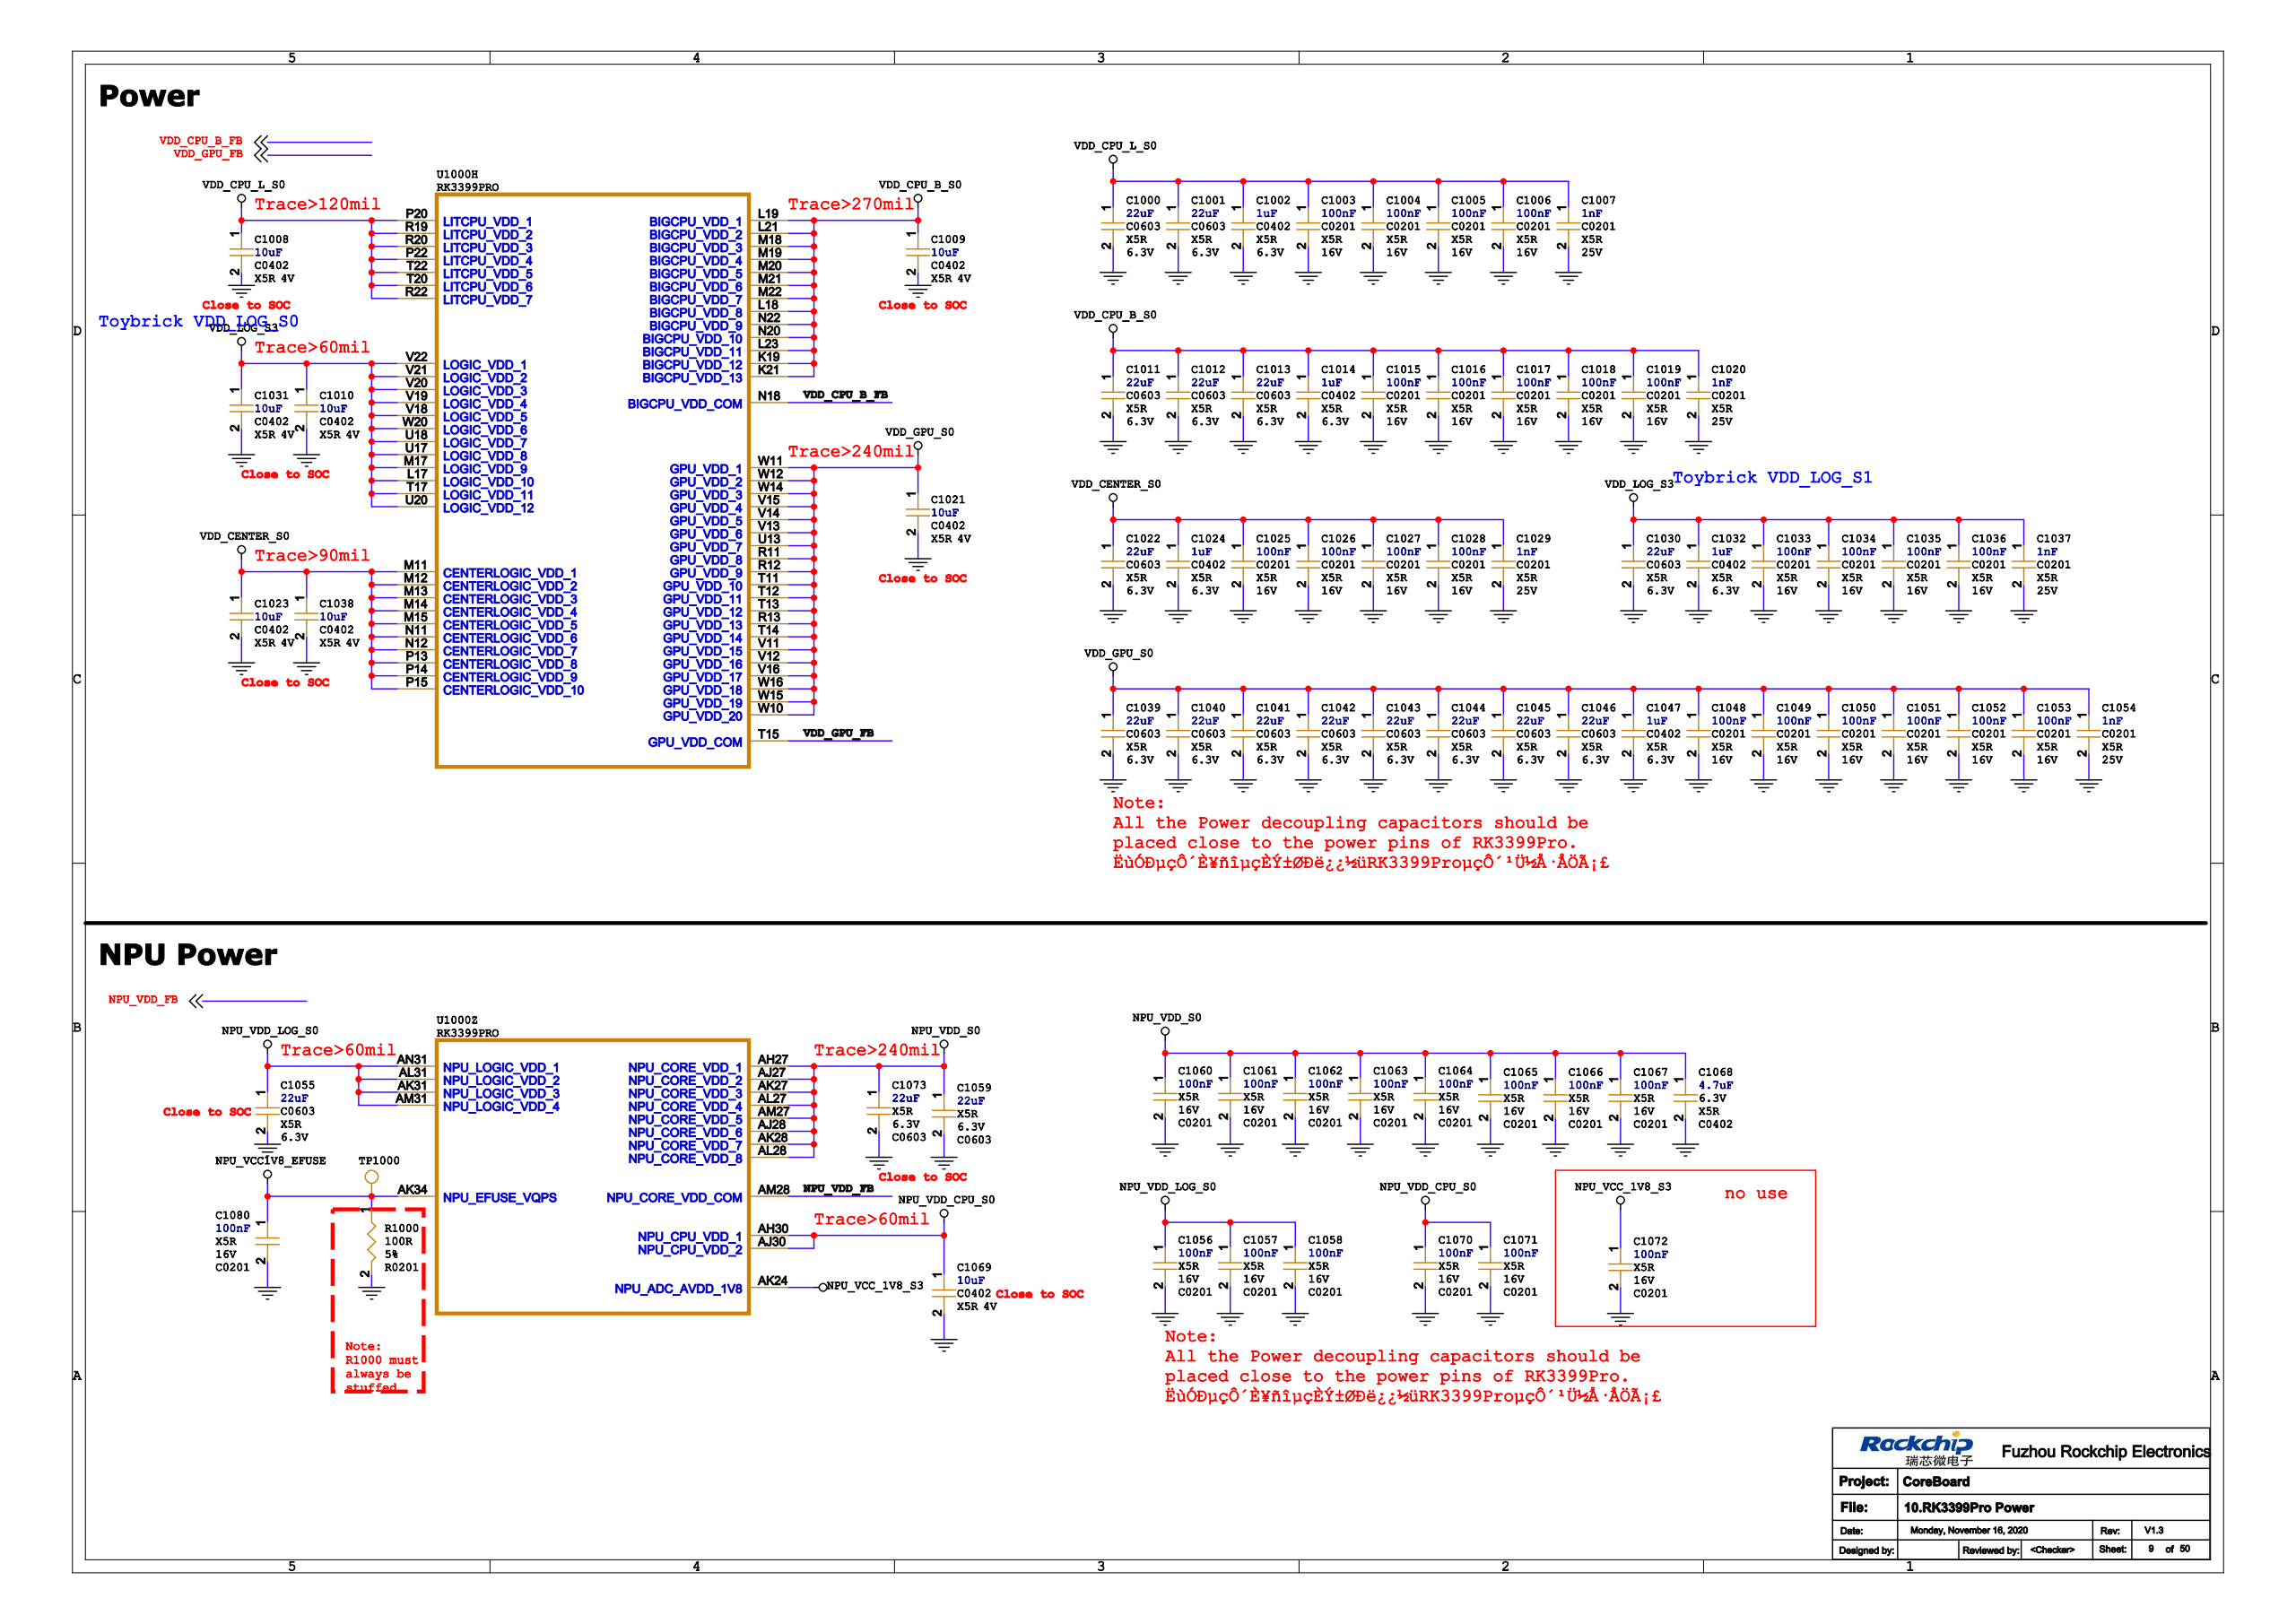Circuit board | Cadence Allegro | 749 parts | 717 nets | one sheet of the schematic
Parts on this sheet (reference | value | footprint):
C1000 | 22uF | C0603
C1001 | 22uF | C0603
C1002 | 1uF | C0402
C1003 | 100nF | C0201
C1004 | 100nF | C0201
C1005 | 100nF | C0201
C1006 | 100nF | C0201
C1007 | 1nF | C0201
C1008 | 10uF | C0402
C1009 | 10uF | C0402
C1010 | 10uF | C0402
C1011 | 22uF | C0603
C1012 | 22uF | C0603
C1013 | 22uF | C0603
C1014 | 1uF | C0402
C1015 | 100nF | C0201
C1016 | 100nF | C0201
C1017 | 100nF | C0201
C1018 | 100nF | C0201
C1019 | 100nF | C0201
C1020 | 1nF | C0201
C1021 | 10uF | C0402
C1022 | 22uF | C0603
C1023 | 10uF | C0402
C1024 | 1uF | C0402
C1025 | 100nF | C0201
C1026 | 100nF | C0201
C1027 | 100nF | C0201
C1028 | 100nF | C0201
C1029 | 1nF | C0201
C1030 | 22uF | C0603
C1031 | 10uF | C0402
C1032 | 1uF | C0402
C1033 | 100nF | C0201
C1034 | 100nF | C0201
C1035 | 100nF | C0201
C1036 | 100nF | C0201
C1037 | 1nF | C0201
C1038 | 10uF | C0402
C1039 | 22uF | C0603
C1040 | 22uF | C0603
C1041 | 22uF | C0603
C1042 | 22uF | C0603
C1043 | 22uF | C0603
C1044 | 22uF | C0603
C1045 | 22uF | C0603
C1046 | 22uF | C0603
C1047 | 1uF | C0402
C1048 | 100nF | C0201
C1049 | 100nF | C0201
C1050 | 100nF | C0201
C1051 | 100nF | C0201
C1052 | 100nF | C0201
C1053 | 100nF | C0201
C1054 | 1nF | C0201
C1055 | 22uF | C0603
C1056 | 100nF | C0201
C1057 | 100nF | C0201
C1058 | 100nF | C0201
C1059 | 22uF | C0603
C1060 | 100nF | C0201
C1061 | 100nF | C0201
C1062 | 100nF | C0201
C1063 | 100nF | C0201
C1064 | 100nF | C0201
C1065 | 100nF | C0201
C1066 | 100nF | C0201
C1067 | 100nF | C0201
C1068 | 4.7uF | C0402
C1069 | 10uF | C0402
C1070 | 100nF | C0201
C1071 | 100nF | C0201
C1072 | 100nF | C0201
C1073 | 22uF | C0603
C1080 | 100nF | C0201
R1000 | 100R | R0201
TP1000 | TP_0.7 | TP_0R70
U1000 | RK3399PRO | BGA1372_27R00X27R00X2R19
Nets of these parts (net: part-pin ...):
GND: C1000-2 C1001-2 C1002-2 C1003-2 C1004-2 C1005-2 C1006-2 C1007-2 C1008-2 C1009-2 C1010-2 C1011-2 C1012-2 C1013-2 C1014-2 C1015-2 C1016-2 C1017-2 C1018-2 C1019-2 C1020-2 C1021-2 C1022-2 C1023-2 C1024-2 C1025-2 C1026-2 C1027-2 C1028-2 C1029-2 C1030-2 C1031-2 C1032-2 C1033-2 C1034-2 C1035-2 C1036-2 C1037-2 C1038-2 C1039-2 C1040-2 C1041-2 C1042-2 C1043-2 C1044-2 C1045-2 C1046-2 C1047-2 C1048-2 C1049-2 C1050-2 C1051-2 C1052-2 C1053-2 C1054-2 C1055-2 C1056-2 C1057-2 C1058-2 C1059-2 C1060-2 C1061-2 C1062-2 C1063-2 C1064-2 C1065-2 C1066-2 C1067-2 C1068-2 C1069-2 C1070-2 C1071-2 C1072-2 C1073-2 C1080-2 R1000-2
VDD_LOG_S3: C1010-1 C1030-1 C1031-1 C1032-1 C1033-1 C1034-1 C1035-1 C1036-1 C1037-1 U1000-L17 U1000-M17 U1000-T17 U1000-U17 U1000-U18 U1000-U20 U1000-V18 U1000-V19 U1000-V20 U1000-V21 U1000-V22 U1000-W20
NPU_VDD_LOG_S0: C1055-1 C1056-1 C1057-1 C1058-1 U1000-AK31 U1000-AL31 U1000-AM31 U1000-AN31
VDD_CENTER_S0: C1022-1 C1023-1 C1024-1 C1025-1 C1026-1 C1027-1 C1028-1 C1029-1 C1038-1 U1000-M11 U1000-M12 U1000-M13 U1000-M14 U1000-M15 U1000-N11 U1000-N12 U1000-P13 U1000-P14 U1000-P15
VDD_CPU_L_S0: C1000-1 C1001-1 C1002-1 C1003-1 C1004-1 C1005-1 C1006-1 C1007-1 C1008-1 U1000-P20 U1000-P22 U1000-R19 U1000-R20 U1000-R22 U1000-T20 U1000-T22
NPU_VDD_CPU_S0: C1069-1 C1070-1 C1071-1 U1000-AH30 U1000-AJ30
NPU_VCC_1V8_S3: C1072-1 U1000-AK24
NPU_VDD_S0: C1059-1 C1060-1 C1061-1 C1062-1 C1063-1 C1064-1 C1065-1 C1066-1 C1067-1 C1068-1 C1073-1 U1000-AH27 U1000-AJ27 U1000-AJ28 U1000-AK27 U1000-AK28 U1000-AL27 U1000-AL28 U1000-AM27
VDD_GPU_S0: C1021-1 C1039-1 C1040-1 C1041-1 C1042-1 C1043-1 C1044-1 C1045-1 C1046-1 C1047-1 C1048-1 C1049-1 C1050-1 C1051-1 C1052-1 C1053-1 C1054-1 U1000-R11 U1000-R12 U1000-R13 U1000-T11 U1000-T12 U1000-T13 U1000-T14 U1000-U13 U1000-V11 U1000-V12 U1000-V13 U1000-V14 U1000-V15 U1000-V16 U1000-W10 U1000-W11 U1000-W12 U1000-W14 U1000-W15 U1000-W16
VDD_CPU_B_S0: C1009-1 C1011-1 C1012-1 C1013-1 C1014-1 C1015-1 C1016-1 C1017-1 C1018-1 C1019-1 C1020-1 U1000-K19 U1000-K21 U1000-L18 U1000-L19 U1000-L21 U1000-L23 U1000-M18 U1000-M19 U1000-M20 U1000-M21 U1000-M22 U1000-N20 U1000-N22
VDD_CPU_B_FB: U1000-N18
VDD_GPU_FB: U1000-T15
NPU_VDD_FB: U1000-AM28
NPU_VCC1V8_EFUSE: C1080-1 R1000-1 TP1000-1 U1000-AK34